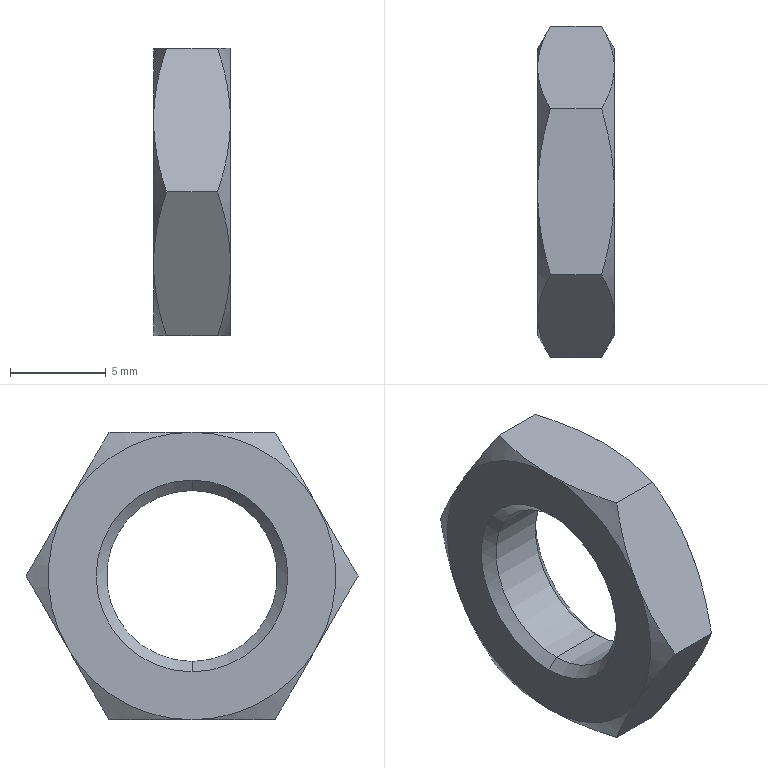Part | STEP file | QA-HI_N-M10x1.0_3 | 1 solid | 26 faces | box 4 x 17.321 x 15 mm | volume 513.744 mm3 | cone 16 | plane 8 | cylinder 2 | commonest cylinder face diameters 8.917 x2